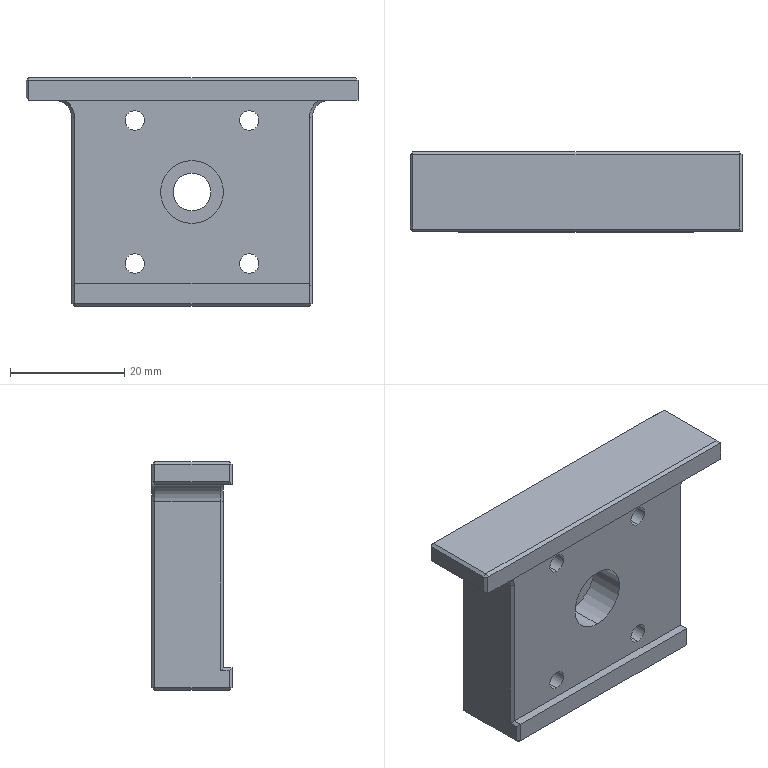Part | STEP file | ND25021-01-JDKM-12-TL | 1 solid | 76 faces | box 58 x 14 x 40 mm | volume 20081 mm3 | plane 48 | cylinder 24 | cone 4 | commonest cylinder face diameters 3.4 x8 6.5 x8 6 x2 6.6 x2 11 x2 20 x2